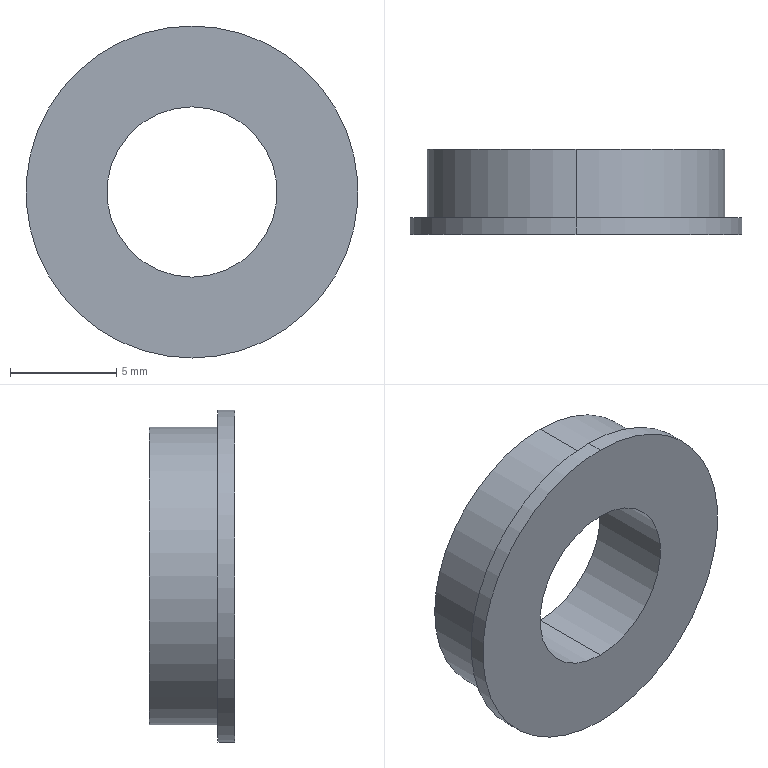Part | STEP file | Bearing 814 | 1 solid | 15 faces | box 15.6 x 4 x 15.6 mm | volume 433.486 mm3 | cylinder 10 | plane 5 | commonest cylinder face diameters 8 x2 9.644 x2 11.88 x2 14 x2 15.6 x2
STEP:
#1=CARTESIAN_POINT('',(0.,0.,0.));
#2=DIRECTION('',(0.,0.,1.));
#3=DIRECTION('',(1.,0.,0.));
#4=AXIS2_PLACEMENT_3D('',#1,#2,#3);
#5=CARTESIAN_POINT('',(0.,0.78,-7.8));
#6=VERTEX_POINT('',#5);
#7=CARTESIAN_POINT('',(0.,0.78,7.8));
#8=VERTEX_POINT('',#7);
#9=CARTESIAN_POINT('',(0.,0.78,0.));
#10=DIRECTION('',(0.,-1.,0.));
#11=DIRECTION('',(0.,0.,-1.));
#12=AXIS2_PLACEMENT_3D('',#9,#10,#11);
#13=CIRCLE('',#12,7.8);
#14=CARTESIAN_POINT('',(0.,0.,0.));
#15=DIRECTION('',(0.,-1.,0.));
#16=DIRECTION('',(0.,0.,-1.));
#17=AXIS2_PLACEMENT_3D('',#14,#15,#16);
#18=CYLINDRICAL_SURFACE('',#17,7.8);
#19=CARTESIAN_POINT('',(0.,-0.78));
#20=DIRECTION('',(1.,0.));
#21=VECTOR('',#20,1.);
#22=LINE('',#19,#21);
#23=(GEOMETRIC_REPRESENTATION_CONTEXT(2)PARAMETRIC_REPRESENTATION_CONTEXT()REPRESENTATION_CONTEXT('',''));
#24=DEFINITIONAL_REPRESENTATION('',(#22),#23);
#25=PCURVE('',#18,#24);
#26=CARTESIAN_POINT('',(7.,0.78,0.));
#27=DIRECTION('',(0.,1.,0.));
#28=DIRECTION('',(0.,0.,1.));
#29=AXIS2_PLACEMENT_3D('',#26,#27,#28);
#30=PLANE('',#29);
#31=CARTESIAN_POINT('',(-7.8,-7.));
#32=CARTESIAN_POINT('',(-7.8,6.51));
#33=CARTESIAN_POINT('',(3.9,-0.245));
#34=CARTESIAN_POINT('',(15.6,-7.));
#35=CARTESIAN_POINT('',(3.9,-13.755));
#36=CARTESIAN_POINT('',(-7.8,-20.51));
#37=CARTESIAN_POINT('',(-7.8,-7.));
#38=(BOUNDED_CURVE()B_SPLINE_CURVE(2,(#31,#32,#33,#34,#35,#36,#37),.UNSPECIFIED.,.T.,.F.)B_SPLINE_CURVE_WITH_KNOTS((1,2,2,2,2,1),(-2.094,0.,2.094,4.189,6.283,8.378),.UNSPECIFIED.)CURVE()GEOMETRIC_REPRESENTATION_ITEM()RATIONAL_B_SPLINE_CURVE((1.,0.5,1.,0.5,1.,0.5,1.))REPRESENTATION_ITEM(''));
#39=(GEOMETRIC_REPRESENTATION_CONTEXT(2)PARAMETRIC_REPRESENTATION_CONTEXT()REPRESENTATION_CONTEXT('',''));
#40=DEFINITIONAL_REPRESENTATION('',(#38),#39);
#41=PCURVE('',#30,#40);
#42=SURFACE_CURVE('',#13,(#25,#41),.PCURVE_S1.);
#43=EDGE_CURVE('',#6,#8,#42,.T.);
#44=ORIENTED_EDGE('',*,*,#43,.T.);
#45=CARTESIAN_POINT('',(0.,0.,7.8));
#46=VERTEX_POINT('',#45);
#47=CARTESIAN_POINT('',(0.,0.,7.8));
#48=DIRECTION('',(0.,-1.,0.));
#49=VECTOR('',#48,1.);
#50=LINE('',#47,#49);
#51=CARTESIAN_POINT('',(3.142,0.));
#52=DIRECTION('',(0.,1.));
#53=VECTOR('',#52,1.);
#54=LINE('',#51,#53);
#55=(GEOMETRIC_REPRESENTATION_CONTEXT(2)PARAMETRIC_REPRESENTATION_CONTEXT()REPRESENTATION_CONTEXT('',''));
#56=DEFINITIONAL_REPRESENTATION('',(#54),#55);
#57=PCURVE('',#18,#56);
#58=CARTESIAN_POINT('',(0.,0.,0.));
#59=DIRECTION('',(0.,-1.,0.));
#60=DIRECTION('',(0.,0.,-1.));
#61=AXIS2_PLACEMENT_3D('',#58,#59,#60);
#62=CYLINDRICAL_SURFACE('',#61,7.8);
#63=CARTESIAN_POINT('',(3.142,0.));
#64=DIRECTION('',(0.,1.));
#65=VECTOR('',#64,1.);
#66=LINE('',#63,#65);
#67=(GEOMETRIC_REPRESENTATION_CONTEXT(2)PARAMETRIC_REPRESENTATION_CONTEXT()REPRESENTATION_CONTEXT('',''));
#68=DEFINITIONAL_REPRESENTATION('',(#66),#67);
#69=PCURVE('',#62,#68);
#70=SURFACE_CURVE('',#50,(#57,#69),.PCURVE_S1.);
#71=EDGE_CURVE('',#8,#46,#70,.T.);
#72=ORIENTED_EDGE('',*,*,#71,.T.);
#73=CARTESIAN_POINT('',(0.,0.,-7.8));
#74=VERTEX_POINT('',#73);
#75=CARTESIAN_POINT('',(0.,0.,0.));
#76=DIRECTION('',(0.,-1.,0.));
#77=DIRECTION('',(0.,0.,-1.));
#78=AXIS2_PLACEMENT_3D('',#75,#76,#77);
#79=CIRCLE('',#78,7.8);
#80=CARTESIAN_POINT('',(0.,0.));
#81=DIRECTION('',(1.,0.));
#82=VECTOR('',#81,1.);
#83=LINE('',#80,#82);
#84=(GEOMETRIC_REPRESENTATION_CONTEXT(2)PARAMETRIC_REPRESENTATION_CONTEXT()REPRESENTATION_CONTEXT('',''));
#85=DEFINITIONAL_REPRESENTATION('',(#83),#84);
#86=PCURVE('',#18,#85);
#87=CARTESIAN_POINT('',(7.8,0.,0.));
#88=DIRECTION('',(0.,-1.,0.));
#89=DIRECTION('',(0.,0.,-1.));
#90=AXIS2_PLACEMENT_3D('',#87,#88,#89);
#91=PLANE('',#90);
#92=CARTESIAN_POINT('',(0.,-7.8));
#93=DIRECTION('',(1.,0.));
#94=AXIS2_PLACEMENT_2D('',#92,#93);
#95=CIRCLE('',#94,7.8);
#96=(GEOMETRIC_REPRESENTATION_CONTEXT(2)PARAMETRIC_REPRESENTATION_CONTEXT()REPRESENTATION_CONTEXT('',''));
#97=DEFINITIONAL_REPRESENTATION('',(#95),#96);
#98=PCURVE('',#91,#97);
#99=SURFACE_CURVE('',#79,(#86,#98),.PCURVE_S1.);
#100=EDGE_CURVE('',#74,#46,#99,.T.);
#101=ORIENTED_EDGE('',*,*,#100,.F.);
#102=CARTESIAN_POINT('',(0.,0.,-7.8));
#103=DIRECTION('',(0.,-1.,0.));
#104=VECTOR('',#103,1.);
#105=LINE('',#102,#104);
#106=CARTESIAN_POINT('',(0.,0.));
#107=DIRECTION('',(0.,1.));
#108=VECTOR('',#107,1.);
#109=LINE('',#106,#108);
#110=(GEOMETRIC_REPRESENTATION_CONTEXT(2)PARAMETRIC_REPRESENTATION_CONTEXT()REPRESENTATION_CONTEXT('',''));
#111=DEFINITIONAL_REPRESENTATION('',(#109),#110);
#112=PCURVE('',#18,#111);
#113=CARTESIAN_POINT('',(6.283,0.));
#114=DIRECTION('',(0.,1.));
#115=VECTOR('',#114,1.);
#116=LINE('',#113,#115);
#117=(GEOMETRIC_REPRESENTATION_CONTEXT(2)PARAMETRIC_REPRESENTATION_CONTEXT()REPRESENTATION_CONTEXT('',''));
#118=DEFINITIONAL_REPRESENTATION('',(#116),#117);
#119=PCURVE('',#62,#118);
#120=SURFACE_CURVE('',#105,(#112,#119),.PCURVE_S1.);
#121=EDGE_CURVE('',#6,#74,#120,.T.);
#122=ORIENTED_EDGE('',*,*,#121,.F.);
#123=EDGE_LOOP('',(#44,#72,#101,#122));
#124=FACE_BOUND('',#123,.T.);
#125=ADVANCED_FACE('',(#124),#18,.T.);
#126=CARTESIAN_POINT('',(0.,4.,-7.));
#127=VERTEX_POINT('',#126);
#128=CARTESIAN_POINT('',(0.,4.,7.));
#129=VERTEX_POINT('',#128);
#130=CARTESIAN_POINT('',(0.,4.,0.));
#131=DIRECTION('',(0.,-1.,0.));
#132=DIRECTION('',(0.,0.,-1.));
#133=AXIS2_PLACEMENT_3D('',#130,#131,#132);
#134=CIRCLE('',#133,7.);
#135=CARTESIAN_POINT('',(0.,0.,0.));
#136=DIRECTION('',(0.,-1.,0.));
#137=DIRECTION('',(0.,0.,-1.));
#138=AXIS2_PLACEMENT_3D('',#135,#136,#137);
#139=CYLINDRICAL_SURFACE('',#138,7.);
#140=CARTESIAN_POINT('',(0.,-4.));
#141=DIRECTION('',(1.,0.));
#142=VECTOR('',#141,1.);
#143=LINE('',#140,#142);
#144=(GEOMETRIC_REPRESENTATION_CONTEXT(2)PARAMETRIC_REPRESENTATION_CONTEXT()REPRESENTATION_CONTEXT('',''));
#145=DEFINITIONAL_REPRESENTATION('',(#143),#144);
#146=PCURVE('',#139,#145);
#147=CARTESIAN_POINT('',(5.94,4.,0.));
#148=DIRECTION('',(0.,1.,0.));
#149=DIRECTION('',(0.,0.,1.));
#150=AXIS2_PLACEMENT_3D('',#147,#148,#149);
#151=PLANE('',#150);
#152=CARTESIAN_POINT('',(-7.,-5.94));
#153=CARTESIAN_POINT('',(-7.,6.184));
#154=CARTESIAN_POINT('',(3.5,0.1221));
#155=CARTESIAN_POINT('',(14.,-5.94));
#156=CARTESIAN_POINT('',(3.5,-12.002));
#157=CARTESIAN_POINT('',(-7.,-18.064));
#158=CARTESIAN_POINT('',(-7.,-5.94));
#159=(BOUNDED_CURVE()B_SPLINE_CURVE(2,(#152,#153,#154,#155,#156,#157,#158),.UNSPECIFIED.,.T.,.F.)B_SPLINE_CURVE_WITH_KNOTS((1,2,2,2,2,1),(-2.094,0.,2.094,4.189,6.283,8.378),.UNSPECIFIED.)CURVE()GEOMETRIC_REPRESENTATION_ITEM()RATIONAL_B_SPLINE_CURVE((1.,0.5,1.,0.5,1.,0.5,1.))REPRESENTATION_ITEM(''));
#160=(GEOMETRIC_REPRESENTATION_CONTEXT(2)PARAMETRIC_REPRESENTATION_CONTEXT()REPRESENTATION_CONTEXT('',''));
#161=DEFINITIONAL_REPRESENTATION('',(#159),#160);
#162=PCURVE('',#151,#161);
#163=SURFACE_CURVE('',#134,(#146,#162),.PCURVE_S1.);
#164=EDGE_CURVE('',#127,#129,#163,.T.);
#165=ORIENTED_EDGE('',*,*,#164,.T.);
#166=CARTESIAN_POINT('',(0.,0.78,7.));
#167=VERTEX_POINT('',#166);
#168=CARTESIAN_POINT('',(0.,0.,7.));
#169=DIRECTION('',(0.,-1.,0.));
#170=VECTOR('',#169,1.);
#171=LINE('',#168,#170);
#172=CARTESIAN_POINT('',(3.142,0.));
#173=DIRECTION('',(0.,1.));
#174=VECTOR('',#173,1.);
#175=LINE('',#172,#174);
#176=(GEOMETRIC_REPRESENTATION_CONTEXT(2)PARAMETRIC_REPRESENTATION_CONTEXT()REPRESENTATION_CONTEXT('',''));
#177=DEFINITIONAL_REPRESENTATION('',(#175),#176);
#178=PCURVE('',#139,#177);
#179=CARTESIAN_POINT('',(0.,0.,0.));
#180=DIRECTION('',(0.,-1.,0.));
#181=DIRECTION('',(0.,0.,-1.));
#182=AXIS2_PLACEMENT_3D('',#179,#180,#181);
#183=CYLINDRICAL_SURFACE('',#182,7.);
#184=CARTESIAN_POINT('',(3.142,0.));
#185=DIRECTION('',(0.,1.));
#186=VECTOR('',#185,1.);
#187=LINE('',#184,#186);
#188=(GEOMETRIC_REPRESENTATION_CONTEXT(2)PARAMETRIC_REPRESENTATION_CONTEXT()REPRESENTATION_CONTEXT('',''));
#189=DEFINITIONAL_REPRESENTATION('',(#187),#188);
#190=PCURVE('',#183,#189);
#191=SURFACE_CURVE('',#171,(#178,#190),.PCURVE_S1.);
#192=EDGE_CURVE('',#129,#167,#191,.T.);
#193=ORIENTED_EDGE('',*,*,#192,.T.);
#194=CARTESIAN_POINT('',(0.,0.78,-7.));
#195=VERTEX_POINT('',#194);
#196=CARTESIAN_POINT('',(0.,0.78,0.));
#197=DIRECTION('',(0.,-1.,0.));
#198=DIRECTION('',(0.,0.,-1.));
#199=AXIS2_PLACEMENT_3D('',#196,#197,#198);
#200=CIRCLE('',#199,7.);
#201=CARTESIAN_POINT('',(0.,-0.78));
#202=DIRECTION('',(1.,0.));
#203=VECTOR('',#202,1.);
#204=LINE('',#201,#203);
#205=(GEOMETRIC_REPRESENTATION_CONTEXT(2)PARAMETRIC_REPRESENTATION_CONTEXT()REPRESENTATION_CONTEXT('',''));
#206=DEFINITIONAL_REPRESENTATION('',(#204),#205);
#207=PCURVE('',#139,#206);
#208=CARTESIAN_POINT('',(-7.,-7.));
#209=CARTESIAN_POINT('',(-7.,5.124));
#210=CARTESIAN_POINT('',(3.5,-0.9378));
#211=CARTESIAN_POINT('',(14.,-7.));
#212=CARTESIAN_POINT('',(3.5,-13.062));
#213=CARTESIAN_POINT('',(-7.,-19.124));
#214=CARTESIAN_POINT('',(-7.,-7.));
#215=(BOUNDED_CURVE()B_SPLINE_CURVE(2,(#208,#209,#210,#211,#212,#213,#214),.UNSPECIFIED.,.T.,.F.)B_SPLINE_CURVE_WITH_KNOTS((1,2,2,2,2,1),(-2.094,0.,2.094,4.189,6.283,8.378),.UNSPECIFIED.)CURVE()GEOMETRIC_REPRESENTATION_ITEM()RATIONAL_B_SPLINE_CURVE((1.,0.5,1.,0.5,1.,0.5,1.))REPRESENTATION_ITEM(''));
#216=(GEOMETRIC_REPRESENTATION_CONTEXT(2)PARAMETRIC_REPRESENTATION_CONTEXT()REPRESENTATION_CONTEXT('',''));
#217=DEFINITIONAL_REPRESENTATION('',(#215),#216);
#218=PCURVE('',#30,#217);
#219=SURFACE_CURVE('',#200,(#207,#218),.PCURVE_S1.);
#220=EDGE_CURVE('',#195,#167,#219,.T.);
#221=ORIENTED_EDGE('',*,*,#220,.F.);
#222=CARTESIAN_POINT('',(0.,0.,-7.));
#223=DIRECTION('',(0.,-1.,0.));
#224=VECTOR('',#223,1.);
#225=LINE('',#222,#224);
#226=CARTESIAN_POINT('',(0.,0.));
#227=DIRECTION('',(0.,1.));
#228=VECTOR('',#227,1.);
#229=LINE('',#226,#228);
#230=(GEOMETRIC_REPRESENTATION_CONTEXT(2)PARAMETRIC_REPRESENTATION_CONTEXT()REPRESENTATION_CONTEXT('',''));
#231=DEFINITIONAL_REPRESENTATION('',(#229),#230);
#232=PCURVE('',#139,#231);
#233=CARTESIAN_POINT('',(6.283,0.));
#234=DIRECTION('',(0.,1.));
#235=VECTOR('',#234,1.);
#236=LINE('',#233,#235);
#237=(GEOMETRIC_REPRESENTATION_CONTEXT(2)PARAMETRIC_REPRESENTATION_CONTEXT()REPRESENTATION_CONTEXT('',''));
#238=DEFINITIONAL_REPRESENTATION('',(#236),#237);
#239=PCURVE('',#183,#238);
#240=SURFACE_CURVE('',#225,(#232,#239),.PCURVE_S1.);
#241=EDGE_CURVE('',#127,#195,#240,.T.);
#242=ORIENTED_EDGE('',*,*,#241,.F.);
#243=EDGE_LOOP('',(#165,#193,#221,#242));
#244=FACE_BOUND('',#243,.T.);
#245=ADVANCED_FACE('',(#244),#139,.T.);
#246=CARTESIAN_POINT('',(0.,4.,-5.94));
#247=VERTEX_POINT('',#246);
#248=CARTESIAN_POINT('',(0.,3.73,-5.94));
#249=VERTEX_POINT('',#248);
#250=CARTESIAN_POINT('',(0.,0.,-5.94));
#251=DIRECTION('',(0.,-1.,0.));
#252=VECTOR('',#251,1.);
#253=LINE('',#250,#252);
#254=CARTESIAN_POINT('',(0.,0.,0.));
#255=DIRECTION('',(0.,-1.,0.));
#256=DIRECTION('',(0.,0.,-1.));
#257=AXIS2_PLACEMENT_3D('',#254,#255,#256);
#258=CYLINDRICAL_SURFACE('',#257,5.94);
#259=CARTESIAN_POINT('',(6.283,0.));
#260=DIRECTION('',(0.,1.));
#261=VECTOR('',#260,1.);
#262=LINE('',#259,#261);
#263=(GEOMETRIC_REPRESENTATION_CONTEXT(2)PARAMETRIC_REPRESENTATION_CONTEXT()REPRESENTATION_CONTEXT('',''));
#264=DEFINITIONAL_REPRESENTATION('',(#262),#263);
#265=PCURVE('',#258,#264);
#266=CARTESIAN_POINT('',(0.,0.,0.));
#267=DIRECTION('',(0.,-1.,0.));
#268=DIRECTION('',(0.,0.,-1.));
#269=AXIS2_PLACEMENT_3D('',#266,#267,#268);
#270=CYLINDRICAL_SURFACE('',#269,5.94);
#271=CARTESIAN_POINT('',(0.,0.));
#272=DIRECTION('',(0.,1.));
#273=VECTOR('',#272,1.);
#274=LINE('',#271,#273);
#275=(GEOMETRIC_REPRESENTATION_CONTEXT(2)PARAMETRIC_REPRESENTATION_CONTEXT()REPRESENTATION_CONTEXT('',''));
#276=DEFINITIONAL_REPRESENTATION('',(#274),#275);
#277=PCURVE('',#270,#276);
#278=SURFACE_CURVE('',#253,(#265,#277),.PCURVE_S1.);
#279=EDGE_CURVE('',#247,#249,#278,.T.);
#280=ORIENTED_EDGE('',*,*,#279,.T.);
#281=CARTESIAN_POINT('',(0.,3.73,5.94));
#282=VERTEX_POINT('',#281);
#283=CARTESIAN_POINT('',(0.,3.73,0.));
#284=DIRECTION('',(0.,-1.,0.));
#285=DIRECTION('',(0.,0.,-1.));
#286=AXIS2_PLACEMENT_3D('',#283,#284,#285);
#287=CIRCLE('',#286,5.94);
#288=CARTESIAN_POINT('',(0.,-3.73));
#289=DIRECTION('',(1.,0.));
#290=VECTOR('',#289,1.);
#291=LINE('',#288,#290);
#292=(GEOMETRIC_REPRESENTATION_CONTEXT(2)PARAMETRIC_REPRESENTATION_CONTEXT()REPRESENTATION_CONTEXT('',''));
#293=DEFINITIONAL_REPRESENTATION('',(#291),#292);
#294=PCURVE('',#258,#293);
#295=CARTESIAN_POINT('',(5.383,3.73,0.));
#296=DIRECTION('',(0.,1.,0.));
#297=DIRECTION('',(0.,0.,1.));
#298=AXIS2_PLACEMENT_3D('',#295,#296,#297);
#299=PLANE('',#298);
#300=CARTESIAN_POINT('',(-5.94,-5.383));
#301=CARTESIAN_POINT('',(-5.94,4.906));
#302=CARTESIAN_POINT('',(2.97,-0.2387));
#303=CARTESIAN_POINT('',(11.88,-5.383));
#304=CARTESIAN_POINT('',(2.97,-10.527));
#305=CARTESIAN_POINT('',(-5.94,-15.672));
#306=CARTESIAN_POINT('',(-5.94,-5.383));
#307=(BOUNDED_CURVE()B_SPLINE_CURVE(2,(#300,#301,#302,#303,#304,#305,#306),.UNSPECIFIED.,.T.,.F.)B_SPLINE_CURVE_WITH_KNOTS((1,2,2,2,2,1),(-2.094,0.,2.094,4.189,6.283,8.378),.UNSPECIFIED.)CURVE()GEOMETRIC_REPRESENTATION_ITEM()RATIONAL_B_SPLINE_CURVE((1.,0.5,1.,0.5,1.,0.5,1.))REPRESENTATION_ITEM(''));
#308=(GEOMETRIC_REPRESENTATION_CONTEXT(2)PARAMETRIC_REPRESENTATION_CONTEXT()REPRESENTATION_CONTEXT('',''));
#309=DEFINITIONAL_REPRESENTATION('',(#307),#308);
#310=PCURVE('',#299,#309);
#311=SURFACE_CURVE('',#287,(#294,#310),.PCURVE_S1.);
#312=EDGE_CURVE('',#282,#249,#311,.T.);
#313=ORIENTED_EDGE('',*,*,#312,.F.);
#314=CARTESIAN_POINT('',(0.,4.,5.94));
#315=VERTEX_POINT('',#314);
#316=CARTESIAN_POINT('',(0.,0.,5.94));
#317=DIRECTION('',(0.,-1.,0.));
#318=VECTOR('',#317,1.);
#319=LINE('',#316,#318);
#320=CARTESIAN_POINT('',(3.142,0.));
#321=DIRECTION('',(0.,1.));
#322=VECTOR('',#321,1.);
#323=LINE('',#320,#322);
#324=(GEOMETRIC_REPRESENTATION_CONTEXT(2)PARAMETRIC_REPRESENTATION_CONTEXT()REPRESENTATION_CONTEXT('',''));
#325=DEFINITIONAL_REPRESENTATION('',(#323),#324);
#326=PCURVE('',#258,#325);
#327=CARTESIAN_POINT('',(3.142,0.));
#328=DIRECTION('',(0.,1.));
#329=VECTOR('',#328,1.);
#330=LINE('',#327,#329);
#331=(GEOMETRIC_REPRESENTATION_CONTEXT(2)PARAMETRIC_REPRESENTATION_CONTEXT()REPRESENTATION_CONTEXT('',''));
#332=DEFINITIONAL_REPRESENTATION('',(#330),#331);
#333=PCURVE('',#270,#332);
#334=SURFACE_CURVE('',#319,(#326,#333),.PCURVE_S1.);
#335=EDGE_CURVE('',#315,#282,#334,.T.);
#336=ORIENTED_EDGE('',*,*,#335,.F.);
#337=CARTESIAN_POINT('',(0.,4.,0.));
#338=DIRECTION('',(0.,-1.,0.));
#339=DIRECTION('',(0.,0.,-1.));
#340=AXIS2_PLACEMENT_3D('',#337,#338,#339);
#341=CIRCLE('',#340,5.94);
#342=CARTESIAN_POINT('',(0.,-4.));
#343=DIRECTION('',(1.,0.));
#344=VECTOR('',#343,1.);
#345=LINE('',#342,#344);
#346=(GEOMETRIC_REPRESENTATION_CONTEXT(2)PARAMETRIC_REPRESENTATION_CONTEXT()REPRESENTATION_CONTEXT('',''));
#347=DEFINITIONAL_REPRESENTATION('',(#345),#346);
#348=PCURVE('',#258,#347);
#349=CARTESIAN_POINT('',(-5.94,-5.94));
#350=CARTESIAN_POINT('',(-5.94,4.348));
#351=CARTESIAN_POINT('',(2.97,-0.7958));
#352=CARTESIAN_POINT('',(11.88,-5.94));
#353=CARTESIAN_POINT('',(2.97,-11.084));
#354=CARTESIAN_POINT('',(-5.94,-16.229));
#355=CARTESIAN_POINT('',(-5.94,-5.94));
#356=(BOUNDED_CURVE()B_SPLINE_CURVE(2,(#349,#350,#351,#352,#353,#354,#355),.UNSPECIFIED.,.T.,.F.)B_SPLINE_CURVE_WITH_KNOTS((1,2,2,2,2,1),(-2.094,0.,2.094,4.189,6.283,8.378),.UNSPECIFIED.)CURVE()GEOMETRIC_REPRESENTATION_ITEM()RATIONAL_B_SPLINE_CURVE((1.,0.5,1.,0.5,1.,0.5,1.))REPRESENTATION_ITEM(''));
#357=(GEOMETRIC_REPRESENTATION_CONTEXT(2)PARAMETRIC_REPRESENTATION_CONTEXT()REPRESENTATION_CONTEXT('',''));
#358=DEFINITIONAL_REPRESENTATION('',(#356),#357);
#359=PCURVE('',#151,#358);
#360=SURFACE_CURVE('',#341,(#348,#359),.PCURVE_S1.);
#361=EDGE_CURVE('',#315,#247,#360,.T.);
#362=ORIENTED_EDGE('',*,*,#361,.T.);
#363=EDGE_LOOP('',(#280,#313,#336,#362));
#364=FACE_BOUND('',#363,.F.);
#365=ADVANCED_FACE('',(#364),#258,.F.);
#366=CARTESIAN_POINT('',(0.,4.,-4.822));
#367=VERTEX_POINT('',#366);
#368=CARTESIAN_POINT('',(0.,4.,4.822));
#369=VERTEX_POINT('',#368);
#370=CARTESIAN_POINT('',(0.,4.,0.));
#371=DIRECTION('',(0.,-1.,0.));
#372=DIRECTION('',(0.,0.,-1.));
#373=AXIS2_PLACEMENT_3D('',#370,#371,#372);
#374=CIRCLE('',#373,4.822);
#375=CARTESIAN_POINT('',(0.,0.,0.));
#376=DIRECTION('',(0.,-1.,0.));
#377=DIRECTION('',(0.,0.,-1.));
#378=AXIS2_PLACEMENT_3D('',#375,#376,#377);
#379=CYLINDRICAL_SURFACE('',#378,4.822);
#380=CARTESIAN_POINT('',(0.,-4.));
#381=DIRECTION('',(1.,0.));
#382=VECTOR('',#381,1.);
#383=LINE('',#380,#382);
#384=(GEOMETRIC_REPRESENTATION_CONTEXT(2)PARAMETRIC_REPRESENTATION_CONTEXT()REPRESENTATION_CONTEXT('',''));
#385=DEFINITIONAL_REPRESENTATION('',(#383),#384);
#386=PCURVE('',#379,#385);
#387=CARTESIAN_POINT('',(4.,4.,0.));
#388=DIRECTION('',(0.,1.,0.));
#389=DIRECTION('',(0.,0.,1.));
#390=AXIS2_PLACEMENT_3D('',#387,#388,#389);
#391=PLANE('',#390);
#392=CARTESIAN_POINT('',(-4.822,-4.));
#393=CARTESIAN_POINT('',(-4.822,4.352));
#394=CARTESIAN_POINT('',(2.411,0.1758));
#395=CARTESIAN_POINT('',(9.644,-4.));
#396=CARTESIAN_POINT('',(2.411,-8.176));
#397=CARTESIAN_POINT('',(-4.822,-12.352));
#398=CARTESIAN_POINT('',(-4.822,-4.));
#399=(BOUNDED_CURVE()B_SPLINE_CURVE(2,(#392,#393,#394,#395,#396,#397,#398),.UNSPECIFIED.,.T.,.F.)B_SPLINE_CURVE_WITH_KNOTS((1,2,2,2,2,1),(-2.094,0.,2.094,4.189,6.283,8.378),.UNSPECIFIED.)CURVE()GEOMETRIC_REPRESENTATION_ITEM()RATIONAL_B_SPLINE_CURVE((1.,0.5,1.,0.5,1.,0.5,1.))REPRESENTATION_ITEM(''));
#400=(GEOMETRIC_REPRESENTATION_CONTEXT(2)PARAMETRIC_REPRESENTATION_CONTEXT()REPRESENTATION_CONTEXT('',''));
#401=DEFINITIONAL_REPRESENTATION('',(#399),#400);
#402=PCURVE('',#391,#401);
#403=SURFACE_CURVE('',#374,(#386,#402),.PCURVE_S1.);
#404=EDGE_CURVE('',#367,#369,#403,.T.);
#405=ORIENTED_EDGE('',*,*,#404,.T.);
#406=CARTESIAN_POINT('',(0.,3.73,4.822));
#407=VERTEX_POINT('',#406);
#408=CARTESIAN_POINT('',(0.,0.,4.822));
#409=DIRECTION('',(0.,-1.,0.));
#410=VECTOR('',#409,1.);
#411=LINE('',#408,#410);
#412=CARTESIAN_POINT('',(3.142,0.));
#413=DIRECTION('',(0.,1.));
#414=VECTOR('',#413,1.);
#415=LINE('',#412,#414);
#416=(GEOMETRIC_REPRESENTATION_CONTEXT(2)PARAMETRIC_REPRESENTATION_CONTEXT()REPRESENTATION_CONTEXT('',''));
#417=DEFINITIONAL_REPRESENTATION('',(#415),#416);
#418=PCURVE('',#379,#417);
#419=CARTESIAN_POINT('',(0.,0.,0.));
#420=DIRECTION('',(0.,-1.,0.));
#421=DIRECTION('',(0.,0.,-1.));
#422=AXIS2_PLACEMENT_3D('',#419,#420,#421);
#423=CYLINDRICAL_SURFACE('',#422,4.822);
#424=CARTESIAN_POINT('',(3.142,0.));
#425=DIRECTION('',(0.,1.));
#426=VECTOR('',#425,1.);
#427=LINE('',#424,#426);
#428=(GEOMETRIC_REPRESENTATION_CONTEXT(2)PARAMETRIC_REPRESENTATION_CONTEXT()REPRESENTATION_CONTEXT('',''));
#429=DEFINITIONAL_REPRESENTATION('',(#427),#428);
#430=PCURVE('',#423,#429);
#431=SURFACE_CURVE('',#411,(#418,#430),.PCURVE_S1.);
#432=EDGE_CURVE('',#369,#407,#431,.T.);
#433=ORIENTED_EDGE('',*,*,#432,.T.);
#434=CARTESIAN_POINT('',(0.,3.73,-4.822));
#435=VERTEX_POINT('',#434);
#436=CARTESIAN_POINT('',(0.,3.73,0.));
#437=DIRECTION('',(0.,-1.,0.));
#438=DIRECTION('',(0.,0.,-1.));
#439=AXIS2_PLACEMENT_3D('',#436,#437,#438);
#440=CIRCLE('',#439,4.822);
#441=CARTESIAN_POINT('',(0.,-3.73));
#442=DIRECTION('',(1.,0.));
#443=VECTOR('',#442,1.);
#444=LINE('',#441,#443);
#445=(GEOMETRIC_REPRESENTATION_CONTEXT(2)PARAMETRIC_REPRESENTATION_CONTEXT()REPRESENTATION_CONTEXT('',''));
#446=DEFINITIONAL_REPRESENTATION('',(#444),#445);
#447=PCURVE('',#379,#446);
#448=CARTESIAN_POINT('',(-4.822,-5.383));
#449=CARTESIAN_POINT('',(-4.822,2.969));
#450=CARTESIAN_POINT('',(2.411,-1.207));
#451=CARTESIAN_POINT('',(9.644,-5.383));
#452=CARTESIAN_POINT('',(2.411,-9.559));
#453=CARTESIAN_POINT('',(-4.822,-13.735));
#454=CARTESIAN_POINT('',(-4.822,-5.383));
#455=(BOUNDED_CURVE()B_SPLINE_CURVE(2,(#448,#449,#450,#451,#452,#453,#454),.UNSPECIFIED.,.T.,.F.)B_SPLINE_CURVE_WITH_KNOTS((1,2,2,2,2,1),(-2.094,0.,2.094,4.189,6.283,8.378),.UNSPECIFIED.)CURVE()GEOMETRIC_REPRESENTATION_ITEM()RATIONAL_B_SPLINE_CURVE((1.,0.5,1.,0.5,1.,0.5,1.))REPRESENTATION_ITEM(''));
#456=(GEOMETRIC_REPRESENTATION_CONTEXT(2)PARAMETRIC_REPRESENTATION_CONTEXT()REPRESENTATION_CONTEXT('',''));
#457=DEFINITIONAL_REPRESENTATION('',(#455),#456);
#458=PCURVE('',#299,#457);
#459=SURFACE_CURVE('',#440,(#447,#458),.PCURVE_S1.);
#460=EDGE_CURVE('',#435,#407,#459,.T.);
#461=ORIENTED_EDGE('',*,*,#460,.F.);
#462=CARTESIAN_POINT('',(0.,0.,-4.822));
#463=DIRECTION('',(0.,-1.,0.));
#464=VECTOR('',#463,1.);
#465=LINE('',#462,#464);
#466=CARTESIAN_POINT('',(0.,0.));
#467=DIRECTION('',(0.,1.));
#468=VECTOR('',#467,1.);
#469=LINE('',#466,#468);
#470=(GEOMETRIC_REPRESENTATION_CONTEXT(2)PARAMETRIC_REPRESENTATION_CONTEXT()REPRESENTATION_CONTEXT('',''));
#471=DEFINITIONAL_REPRESENTATION('',(#469),#470);
#472=PCURVE('',#379,#471);
#473=CARTESIAN_POINT('',(6.283,0.));
#474=DIRECTION('',(0.,1.));
#475=VECTOR('',#474,1.);
#476=LINE('',#473,#475);
#477=(GEOMETRIC_REPRESENTATION_CONTEXT(2)PARAMETRIC_REPRESENTATION_CONTEXT()REPRESENTATION_CONTEXT('',''));
#478=DEFINITIONAL_REPRESENTATION('',(#476),#477);
#479=PCURVE('',#423,#478);
#480=SURFACE_CURVE('',#465,(#472,#479),.PCURVE_S1.);
#481=EDGE_CURVE('',#367,#435,#480,.T.);
#482=ORIENTED_EDGE('',*,*,#481,.F.);
#483=EDGE_LOOP('',(#405,#433,#461,#482));
#484=FACE_BOUND('',#483,.T.);
#485=ADVANCED_FACE('',(#484),#379,.T.);
#486=CARTESIAN_POINT('',(0.,4.,-4.));
#487=VERTEX_POINT('',#486);
#488=CARTESIAN_POINT('',(0.,0.,-4.));
#489=VERTEX_POINT('',#488);
#490=CARTESIAN_POINT('',(0.,0.,-4.));
#491=DIRECTION('',(0.,-1.,0.));
#492=VECTOR('',#491,1.);
#493=LINE('',#490,#492);
#494=CARTESIAN_POINT('',(0.,0.,0.));
#495=DIRECTION('',(0.,-1.,0.));
#496=DIRECTION('',(0.,0.,-1.));
#497=AXIS2_PLACEMENT_3D('',#494,#495,#496);
#498=CYLINDRICAL_SURFACE('',#497,4.);
#499=CARTESIAN_POINT('',(6.283,0.));
#500=DIRECTION('',(0.,1.));
#501=VECTOR('',#500,1.);
#502=LINE('',#499,#501);
#503=(GEOMETRIC_REPRESENTATION_CONTEXT(2)PARAMETRIC_REPRESENTATION_CONTEXT()REPRESENTATION_CONTEXT('',''));
#504=DEFINITIONAL_REPRESENTATION('',(#502),#503);
#505=PCURVE('',#498,#504);
#506=CARTESIAN_POINT('',(0.,0.,0.));
#507=DIRECTION('',(0.,-1.,0.));
#508=DIRECTION('',(0.,0.,-1.));
#509=AXIS2_PLACEMENT_3D('',#506,#507,#508);
#510=CYLINDRICAL_SURFACE('',#509,4.);
#511=CARTESIAN_POINT('',(0.,0.));
#512=DIRECTION('',(0.,1.));
#513=VECTOR('',#512,1.);
#514=LINE('',#511,#513);
#515=(GEOMETRIC_REPRESENTATION_CONTEXT(2)PARAMETRIC_REPRESENTATION_CONTEXT()REPRESENTATION_CONTEXT('',''));
#516=DEFINITIONAL_REPRESENTATION('',(#514),#515);
#517=PCURVE('',#510,#516);
#518=SURFACE_CURVE('',#493,(#505,#517),.PCURVE_S1.);
#519=EDGE_CURVE('',#487,#489,#518,.T.);
#520=ORIENTED_EDGE('',*,*,#519,.T.);
#521=CARTESIAN_POINT('',(0.,0.,4.));
#522=VERTEX_POINT('',#521);
#523=CARTESIAN_POINT('',(0.,0.,0.));
#524=DIRECTION('',(0.,-1.,0.));
#525=DIRECTION('',(0.,0.,-1.));
#526=AXIS2_PLACEMENT_3D('',#523,#524,#525);
#527=CIRCLE('',#526,4.);
#528=CARTESIAN_POINT('',(0.,0.));
#529=DIRECTION('',(1.,0.));
#530=VECTOR('',#529,1.);
#531=LINE('',#528,#530);
#532=(GEOMETRIC_REPRESENTATION_CONTEXT(2)PARAMETRIC_REPRESENTATION_CONTEXT()REPRESENTATION_CONTEXT('',''));
#533=DEFINITIONAL_REPRESENTATION('',(#531),#532);
#534=PCURVE('',#498,#533);
#535=CARTESIAN_POINT('',(0.,-7.8));
#536=DIRECTION('',(1.,0.));
#537=AXIS2_PLACEMENT_2D('',#535,#536);
#538=CIRCLE('',#537,4.);
#539=(GEOMETRIC_REPRESENTATION_CONTEXT(2)PARAMETRIC_REPRESENTATION_CONTEXT()REPRESENTATION_CONTEXT('',''));
#540=DEFINITIONAL_REPRESENTATION('',(#538),#539);
#541=PCURVE('',#91,#540);
#542=SURFACE_CURVE('',#527,(#534,#541),.PCURVE_S1.);
#543=EDGE_CURVE('',#522,#489,#542,.T.);
#544=ORIENTED_EDGE('',*,*,#543,.F.);
#545=CARTESIAN_POINT('',(0.,4.,4.));
#546=VERTEX_POINT('',#545);
#547=CARTESIAN_POINT('',(0.,0.,4.));
#548=DIRECTION('',(0.,-1.,0.));
#549=VECTOR('',#548,1.);
#550=LINE('',#547,#549);
#551=CARTESIAN_POINT('',(3.142,0.));
#552=DIRECTION('',(0.,1.));
#553=VECTOR('',#552,1.);
#554=LINE('',#551,#553);
#555=(GEOMETRIC_REPRESENTATION_CONTEXT(2)PARAMETRIC_REPRESENTATION_CONTEXT()REPRESENTATION_CONTEXT('',''));
#556=DEFINITIONAL_REPRESENTATION('',(#554),#555);
#557=PCURVE('',#498,#556);
#558=CARTESIAN_POINT('',(3.142,0.));
#559=DIRECTION('',(0.,1.));
#560=VECTOR('',#559,1.);
#561=LINE('',#558,#560);
#562=(GEOMETRIC_REPRESENTATION_CONTEXT(2)PARAMETRIC_REPRESENTATION_CONTEXT()REPRESENTATION_CONTEXT('',''));
#563=DEFINITIONAL_REPRESENTATION('',(#561),#562);
#564=PCURVE('',#510,#563);
#565=SURFACE_CURVE('',#550,(#557,#564),.PCURVE_S1.);
#566=EDGE_CURVE('',#546,#522,#565,.T.);
#567=ORIENTED_EDGE('',*,*,#566,.F.);
#568=CARTESIAN_POINT('',(0.,4.,0.));
#569=DIRECTION('',(0.,-1.,0.));
#570=DIRECTION('',(0.,0.,-1.));
#571=AXIS2_PLACEMENT_3D('',#568,#569,#570);
#572=CIRCLE('',#571,4.);
#573=CARTESIAN_POINT('',(0.,-4.));
#574=DIRECTION('',(1.,0.));
#575=VECTOR('',#574,1.);
#576=LINE('',#573,#575);
#577=(GEOMETRIC_REPRESENTATION_CONTEXT(2)PARAMETRIC_REPRESENTATION_CONTEXT()REPRESENTATION_CONTEXT('',''));
#578=DEFINITIONAL_REPRESENTATION('',(#576),#577);
#579=PCURVE('',#498,#578);
#580=CARTESIAN_POINT('',(-4.,-4.));
#581=CARTESIAN_POINT('',(-4.,2.928));
#582=CARTESIAN_POINT('',(2.,-0.5359));
#583=CARTESIAN_POINT('',(8.,-4.));
#584=CARTESIAN_POINT('',(2.,-7.464));
#585=CARTESIAN_POINT('',(-4.,-10.928));
#586=CARTESIAN_POINT('',(-4.,-4.));
#587=(BOUNDED_CURVE()B_SPLINE_CURVE(2,(#580,#581,#582,#583,#584,#585,#586),.UNSPECIFIED.,.T.,.F.)B_SPLINE_CURVE_WITH_KNOTS((1,2,2,2,2,1),(-2.094,0.,2.094,4.189,6.283,8.378),.UNSPECIFIED.)CURVE()GEOMETRIC_REPRESENTATION_ITEM()RATIONAL_B_SPLINE_CURVE((1.,0.5,1.,0.5,1.,0.5,1.))REPRESENTATION_ITEM(''));
#588=(GEOMETRIC_REPRESENTATION_CONTEXT(2)PARAMETRIC_REPRESENTATION_CONTEXT()REPRESENTATION_CONTEXT('',''));
#589=DEFINITIONAL_REPRESENTATION('',(#587),#588);
#590=PCURVE('',#391,#589);
#591=SURFACE_CURVE('',#572,(#579,#590),.PCURVE_S1.);
#592=EDGE_CURVE('',#546,#487,#591,.T.);
#593=ORIENTED_EDGE('',*,*,#592,.T.);
#594=EDGE_LOOP('',(#520,#544,#567,#593));
#595=FACE_BOUND('',#594,.F.);
#596=ADVANCED_FACE('',(#595),#498,.F.);
#597=ORIENTED_EDGE('',*,*,#100,.T.);
#598=CARTESIAN_POINT('',(0.,0.,0.));
#599=DIRECTION('',(0.,-1.,0.));
#600=DIRECTION('',(0.,0.,-1.));
#601=AXIS2_PLACEMENT_3D('',#598,#599,#600);
#602=CIRCLE('',#601,7.8);
#603=CARTESIAN_POINT('',(0.,-7.8));
#604=DIRECTION('',(1.,0.));
#605=AXIS2_PLACEMENT_2D('',#603,#604);
#606=CIRCLE('',#605,7.8);
#607=(GEOMETRIC_REPRESENTATION_CONTEXT(2)PARAMETRIC_REPRESENTATION_CONTEXT()REPRESENTATION_CONTEXT('',''));
#608=DEFINITIONAL_REPRESENTATION('',(#606),#607);
#609=PCURVE('',#91,#608);
#610=CARTESIAN_POINT('',(0.,0.));
#611=DIRECTION('',(1.,0.));
#612=VECTOR('',#611,1.);
#613=LINE('',#610,#612);
#614=(GEOMETRIC_REPRESENTATION_CONTEXT(2)PARAMETRIC_REPRESENTATION_CONTEXT()REPRESENTATION_CONTEXT('',''));
#615=DEFINITIONAL_REPRESENTATION('',(#613),#614);
#616=PCURVE('',#62,#615);
#617=SURFACE_CURVE('',#602,(#609,#616),.PCURVE_S1.);
#618=EDGE_CURVE('',#46,#74,#617,.T.);
#619=ORIENTED_EDGE('',*,*,#618,.T.);
#620=EDGE_LOOP('',(#597,#619));
#621=FACE_BOUND('',#620,.T.);
#622=CARTESIAN_POINT('',(0.,0.,0.));
#623=DIRECTION('',(0.,-1.,0.));
#624=DIRECTION('',(0.,0.,-1.));
#625=AXIS2_PLACEMENT_3D('',#622,#623,#624);
#626=CIRCLE('',#625,4.);
#627=CARTESIAN_POINT('',(0.,-7.8));
#628=DIRECTION('',(1.,0.));
#629=AXIS2_PLACEMENT_2D('',#627,#628);
#630=CIRCLE('',#629,4.);
#631=(GEOMETRIC_REPRESENTATION_CONTEXT(2)PARAMETRIC_REPRESENTATION_CONTEXT()REPRESENTATION_CONTEXT('',''));
#632=DEFINITIONAL_REPRESENTATION('',(#630),#631);
#633=PCURVE('',#91,#632);
#634=CARTESIAN_POINT('',(0.,0.));
#635=DIRECTION('',(1.,0.));
#636=VECTOR('',#635,1.);
#637=LINE('',#634,#636);
#638=(GEOMETRIC_REPRESENTATION_CONTEXT(2)PARAMETRIC_REPRESENTATION_CONTEXT()REPRESENTATION_CONTEXT('',''));
#639=DEFINITIONAL_REPRESENTATION('',(#637),#638);
#640=PCURVE('',#510,#639);
#641=SURFACE_CURVE('',#626,(#633,#640),.PCURVE_S1.);
#642=EDGE_CURVE('',#489,#522,#641,.T.);
#643=ORIENTED_EDGE('',*,*,#642,.F.);
#644=ORIENTED_EDGE('',*,*,#543,.F.);
#645=EDGE_LOOP('',(#643,#644));
#646=FACE_BOUND('',#645,.T.);
#647=ADVANCED_FACE('',(#621,#646),#91,.T.);
#648=ORIENTED_EDGE('',*,*,#642,.F.);
#649=ORIENTED_EDGE('',*,*,#519,.F.);
#650=CARTESIAN_POINT('',(0.,4.,0.));
#651=DIRECTION('',(0.,-1.,0.));
#652=DIRECTION('',(0.,0.,-1.));
#653=AXIS2_PLACEMENT_3D('',#650,#651,#652);
#654=CIRCLE('',#653,4.);
#655=CARTESIAN_POINT('',(0.,-4.));
#656=DIRECTION('',(1.,0.));
#657=VECTOR('',#656,1.);
#658=LINE('',#655,#657);
#659=(GEOMETRIC_REPRESENTATION_CONTEXT(2)PARAMETRIC_REPRESENTATION_CONTEXT()REPRESENTATION_CONTEXT('',''));
#660=DEFINITIONAL_REPRESENTATION('',(#658),#659);
#661=PCURVE('',#510,#660);
#662=CARTESIAN_POINT('',(-4.,-4.));
#663=CARTESIAN_POINT('',(-4.,2.928));
#664=CARTESIAN_POINT('',(2.,-0.5359));
#665=CARTESIAN_POINT('',(8.,-4.));
#666=CARTESIAN_POINT('',(2.,-7.464));
#667=CARTESIAN_POINT('',(-4.,-10.928));
#668=CARTESIAN_POINT('',(-4.,-4.));
#669=(BOUNDED_CURVE()B_SPLINE_CURVE(2,(#662,#663,#664,#665,#666,#667,#668),.UNSPECIFIED.,.T.,.F.)B_SPLINE_CURVE_WITH_KNOTS((1,2,2,2,2,1),(-2.094,0.,2.094,4.189,6.283,8.378),.UNSPECIFIED.)CURVE()GEOMETRIC_REPRESENTATION_ITEM()RATIONAL_B_SPLINE_CURVE((1.,0.5,1.,0.5,1.,0.5,1.))REPRESENTATION_ITEM(''));
#670=(GEOMETRIC_REPRESENTATION_CONTEXT(2)PARAMETRIC_REPRESENTATION_CONTEXT()REPRESENTATION_CONTEXT('',''));
#671=DEFINITIONAL_REPRESENTATION('',(#669),#670);
#672=PCURVE('',#391,#671);
#673=SURFACE_CURVE('',#654,(#661,#672),.PCURVE_S1.);
#674=EDGE_CURVE('',#487,#546,#673,.T.);
#675=ORIENTED_EDGE('',*,*,#674,.T.);
#676=ORIENTED_EDGE('',*,*,#566,.T.);
#677=EDGE_LOOP('',(#648,#649,#675,#676));
#678=FACE_BOUND('',#677,.F.);
#679=ADVANCED_FACE('',(#678),#510,.F.);
#680=ORIENTED_EDGE('',*,*,#674,.T.);
#681=ORIENTED_EDGE('',*,*,#592,.T.);
#682=EDGE_LOOP('',(#680,#681));
#683=FACE_BOUND('',#682,.T.);
#684=ORIENTED_EDGE('',*,*,#404,.F.);
#685=CARTESIAN_POINT('',(0.,4.,0.));
#686=DIRECTION('',(0.,-1.,0.));
#687=DIRECTION('',(0.,0.,-1.));
#688=AXIS2_PLACEMENT_3D('',#685,#686,#687);
#689=CIRCLE('',#688,4.822);
#690=CARTESIAN_POINT('',(-4.822,-4.));
#691=CARTESIAN_POINT('',(-4.822,4.352));
#692=CARTESIAN_POINT('',(2.411,0.1758));
#693=CARTESIAN_POINT('',(9.644,-4.));
#694=CARTESIAN_POINT('',(2.411,-8.176));
#695=CARTESIAN_POINT('',(-4.822,-12.352));
#696=CARTESIAN_POINT('',(-4.822,-4.));
#697=(BOUNDED_CURVE()B_SPLINE_CURVE(2,(#690,#691,#692,#693,#694,#695,#696),.UNSPECIFIED.,.T.,.F.)B_SPLINE_CURVE_WITH_KNOTS((1,2,2,2,2,1),(-2.094,0.,2.094,4.189,6.283,8.378),.UNSPECIFIED.)CURVE()GEOMETRIC_REPRESENTATION_ITEM()RATIONAL_B_SPLINE_CURVE((1.,0.5,1.,0.5,1.,0.5,1.))REPRESENTATION_ITEM(''));
#698=(GEOMETRIC_REPRESENTATION_CONTEXT(2)PARAMETRIC_REPRESENTATION_CONTEXT()REPRESENTATION_CONTEXT('',''));
#699=DEFINITIONAL_REPRESENTATION('',(#697),#698);
#700=PCURVE('',#391,#699);
#701=CARTESIAN_POINT('',(0.,-4.));
#702=DIRECTION('',(1.,0.));
#703=VECTOR('',#702,1.);
#704=LINE('',#701,#703);
#705=(GEOMETRIC_REPRESENTATION_CONTEXT(2)PARAMETRIC_REPRESENTATION_CONTEXT()REPRESENTATION_CONTEXT('',''));
#706=DEFINITIONAL_REPRESENTATION('',(#704),#705);
#707=PCURVE('',#423,#706);
#708=SURFACE_CURVE('',#689,(#700,#707),.PCURVE_S1.);
#709=EDGE_CURVE('',#369,#367,#708,.T.);
#710=ORIENTED_EDGE('',*,*,#709,.F.);
#711=EDGE_LOOP('',(#684,#710));
#712=FACE_BOUND('',#711,.T.);
#713=ADVANCED_FACE('',(#683,#712),#391,.T.);
#714=ORIENTED_EDGE('',*,*,#432,.F.);
#715=ORIENTED_EDGE('',*,*,#709,.T.);
#716=ORIENTED_EDGE('',*,*,#481,.T.);
#717=CARTESIAN_POINT('',(0.,3.73,0.));
#718=DIRECTION('',(0.,-1.,0.));
#719=DIRECTION('',(0.,0.,-1.));
#720=AXIS2_PLACEMENT_3D('',#717,#718,#719);
#721=CIRCLE('',#720,4.822);
#722=CARTESIAN_POINT('',(0.,-3.73));
#723=DIRECTION('',(1.,0.));
#724=VECTOR('',#723,1.);
#725=LINE('',#722,#724);
#726=(GEOMETRIC_REPRESENTATION_CONTEXT(2)PARAMETRIC_REPRESENTATION_CONTEXT()REPRESENTATION_CONTEXT('',''));
#727=DEFINITIONAL_REPRESENTATION('',(#725),#726);
#728=PCURVE('',#423,#727);
#729=CARTESIAN_POINT('',(-4.822,-5.383));
#730=CARTESIAN_POINT('',(-4.822,2.969));
#731=CARTESIAN_POINT('',(2.411,-1.207));
#732=CARTESIAN_POINT('',(9.644,-5.383));
#733=CARTESIAN_POINT('',(2.411,-9.559));
#734=CARTESIAN_POINT('',(-4.822,-13.735));
#735=CARTESIAN_POINT('',(-4.822,-5.383));
#736=(BOUNDED_CURVE()B_SPLINE_CURVE(2,(#729,#730,#731,#732,#733,#734,#735),.UNSPECIFIED.,.T.,.F.)B_SPLINE_CURVE_WITH_KNOTS((1,2,2,2,2,1),(-2.094,0.,2.094,4.189,6.283,8.378),.UNSPECIFIED.)CURVE()GEOMETRIC_REPRESENTATION_ITEM()RATIONAL_B_SPLINE_CURVE((1.,0.5,1.,0.5,1.,0.5,1.))REPRESENTATION_ITEM(''));
#737=(GEOMETRIC_REPRESENTATION_CONTEXT(2)PARAMETRIC_REPRESENTATION_CONTEXT()REPRESENTATION_CONTEXT('',''));
#738=DEFINITIONAL_REPRESENTATION('',(#736),#737);
#739=PCURVE('',#299,#738);
#740=SURFACE_CURVE('',#721,(#728,#739),.PCURVE_S1.);
#741=EDGE_CURVE('',#407,#435,#740,.T.);
#742=ORIENTED_EDGE('',*,*,#741,.F.);
#743=EDGE_LOOP('',(#714,#715,#716,#742));
#744=FACE_BOUND('',#743,.T.);
#745=ADVANCED_FACE('',(#744),#423,.T.);
#746=ORIENTED_EDGE('',*,*,#460,.T.);
#747=ORIENTED_EDGE('',*,*,#741,.T.);
#748=EDGE_LOOP('',(#746,#747));
#749=FACE_BOUND('',#748,.T.);
#750=CARTESIAN_POINT('',(0.,3.73,0.));
#751=DIRECTION('',(0.,-1.,0.));
#752=DIRECTION('',(0.,0.,-1.));
#753=AXIS2_PLACEMENT_3D('',#750,#751,#752);
#754=CIRCLE('',#753,5.94);
#755=CARTESIAN_POINT('',(-5.94,-5.383));
#756=CARTESIAN_POINT('',(-5.94,4.906));
#757=CARTESIAN_POINT('',(2.97,-0.2387));
#758=CARTESIAN_POINT('',(11.88,-5.383));
#759=CARTESIAN_POINT('',(2.97,-10.527));
#760=CARTESIAN_POINT('',(-5.94,-15.672));
#761=CARTESIAN_POINT('',(-5.94,-5.383));
#762=(BOUNDED_CURVE()B_SPLINE_CURVE(2,(#755,#756,#757,#758,#759,#760,#761),.UNSPECIFIED.,.T.,.F.)B_SPLINE_CURVE_WITH_KNOTS((1,2,2,2,2,1),(-2.094,0.,2.094,4.189,6.283,8.378),.UNSPECIFIED.)CURVE()GEOMETRIC_REPRESENTATION_ITEM()RATIONAL_B_SPLINE_CURVE((1.,0.5,1.,0.5,1.,0.5,1.))REPRESENTATION_ITEM(''));
#763=(GEOMETRIC_REPRESENTATION_CONTEXT(2)PARAMETRIC_REPRESENTATION_CONTEXT()REPRESENTATION_CONTEXT('',''));
#764=DEFINITIONAL_REPRESENTATION('',(#762),#763);
#765=PCURVE('',#299,#764);
#766=CARTESIAN_POINT('',(0.,-3.73));
#767=DIRECTION('',(1.,0.));
#768=VECTOR('',#767,1.);
#769=LINE('',#766,#768);
#770=(GEOMETRIC_REPRESENTATION_CONTEXT(2)PARAMETRIC_REPRESENTATION_CONTEXT()REPRESENTATION_CONTEXT('',''));
#771=DEFINITIONAL_REPRESENTATION('',(#769),#770);
#772=PCURVE('',#270,#771);
#773=SURFACE_CURVE('',#754,(#765,#772),.PCURVE_S1.);
#774=EDGE_CURVE('',#249,#282,#773,.T.);
#775=ORIENTED_EDGE('',*,*,#774,.F.);
#776=ORIENTED_EDGE('',*,*,#312,.F.);
#777=EDGE_LOOP('',(#775,#776));
#778=FACE_BOUND('',#777,.T.);
#779=ADVANCED_FACE('',(#749,#778),#299,.T.);
#780=ORIENTED_EDGE('',*,*,#774,.F.);
#781=ORIENTED_EDGE('',*,*,#279,.F.);
#782=CARTESIAN_POINT('',(0.,4.,0.));
#783=DIRECTION('',(0.,-1.,0.));
#784=DIRECTION('',(0.,0.,-1.));
#785=AXIS2_PLACEMENT_3D('',#782,#783,#784);
#786=CIRCLE('',#785,5.94);
#787=CARTESIAN_POINT('',(0.,-4.));
#788=DIRECTION('',(1.,0.));
#789=VECTOR('',#788,1.);
#790=LINE('',#787,#789);
#791=(GEOMETRIC_REPRESENTATION_CONTEXT(2)PARAMETRIC_REPRESENTATION_CONTEXT()REPRESENTATION_CONTEXT('',''));
#792=DEFINITIONAL_REPRESENTATION('',(#790),#791);
#793=PCURVE('',#270,#792);
#794=CARTESIAN_POINT('',(-5.94,-5.94));
#795=CARTESIAN_POINT('',(-5.94,4.348));
#796=CARTESIAN_POINT('',(2.97,-0.7958));
#797=CARTESIAN_POINT('',(11.88,-5.94));
#798=CARTESIAN_POINT('',(2.97,-11.084));
#799=CARTESIAN_POINT('',(-5.94,-16.229));
#800=CARTESIAN_POINT('',(-5.94,-5.94));
#801=(BOUNDED_CURVE()B_SPLINE_CURVE(2,(#794,#795,#796,#797,#798,#799,#800),.UNSPECIFIED.,.T.,.F.)B_SPLINE_CURVE_WITH_KNOTS((1,2,2,2,2,1),(-2.094,0.,2.094,4.189,6.283,8.378),.UNSPECIFIED.)CURVE()GEOMETRIC_REPRESENTATION_ITEM()RATIONAL_B_SPLINE_CURVE((1.,0.5,1.,0.5,1.,0.5,1.))REPRESENTATION_ITEM(''));
#802=(GEOMETRIC_REPRESENTATION_CONTEXT(2)PARAMETRIC_REPRESENTATION_CONTEXT()REPRESENTATION_CONTEXT('',''));
#803=DEFINITIONAL_REPRESENTATION('',(#801),#802);
#804=PCURVE('',#151,#803);
#805=SURFACE_CURVE('',#786,(#793,#804),.PCURVE_S1.);
#806=EDGE_CURVE('',#247,#315,#805,.T.);
#807=ORIENTED_EDGE('',*,*,#806,.T.);
#808=ORIENTED_EDGE('',*,*,#335,.T.);
#809=EDGE_LOOP('',(#780,#781,#807,#808));
#810=FACE_BOUND('',#809,.F.);
#811=ADVANCED_FACE('',(#810),#270,.F.);
#812=ORIENTED_EDGE('',*,*,#806,.T.);
#813=ORIENTED_EDGE('',*,*,#361,.T.);
#814=EDGE_LOOP('',(#812,#813));
#815=FACE_BOUND('',#814,.T.);
#816=ORIENTED_EDGE('',*,*,#164,.F.);
#817=CARTESIAN_POINT('',(0.,4.,0.));
#818=DIRECTION('',(0.,-1.,0.));
#819=DIRECTION('',(0.,0.,-1.));
#820=AXIS2_PLACEMENT_3D('',#817,#818,#819);
#821=CIRCLE('',#820,7.);
#822=CARTESIAN_POINT('',(-7.,-5.94));
#823=CARTESIAN_POINT('',(-7.,6.184));
#824=CARTESIAN_POINT('',(3.5,0.1221));
#825=CARTESIAN_POINT('',(14.,-5.94));
#826=CARTESIAN_POINT('',(3.5,-12.002));
#827=CARTESIAN_POINT('',(-7.,-18.064));
#828=CARTESIAN_POINT('',(-7.,-5.94));
#829=(BOUNDED_CURVE()B_SPLINE_CURVE(2,(#822,#823,#824,#825,#826,#827,#828),.UNSPECIFIED.,.T.,.F.)B_SPLINE_CURVE_WITH_KNOTS((1,2,2,2,2,1),(-2.094,0.,2.094,4.189,6.283,8.378),.UNSPECIFIED.)CURVE()GEOMETRIC_REPRESENTATION_ITEM()RATIONAL_B_SPLINE_CURVE((1.,0.5,1.,0.5,1.,0.5,1.))REPRESENTATION_ITEM(''));
#830=(GEOMETRIC_REPRESENTATION_CONTEXT(2)PARAMETRIC_REPRESENTATION_CONTEXT()REPRESENTATION_CONTEXT('',''));
#831=DEFINITIONAL_REPRESENTATION('',(#829),#830);
#832=PCURVE('',#151,#831);
#833=CARTESIAN_POINT('',(0.,-4.));
#834=DIRECTION('',(1.,0.));
#835=VECTOR('',#834,1.);
#836=LINE('',#833,#835);
#837=(GEOMETRIC_REPRESENTATION_CONTEXT(2)PARAMETRIC_REPRESENTATION_CONTEXT()REPRESENTATION_CONTEXT('',''));
#838=DEFINITIONAL_REPRESENTATION('',(#836),#837);
#839=PCURVE('',#183,#838);
#840=SURFACE_CURVE('',#821,(#832,#839),.PCURVE_S1.);
#841=EDGE_CURVE('',#129,#127,#840,.T.);
#842=ORIENTED_EDGE('',*,*,#841,.F.);
#843=EDGE_LOOP('',(#816,#842));
#844=FACE_BOUND('',#843,.T.);
#845=ADVANCED_FACE('',(#815,#844),#151,.T.);
#846=ORIENTED_EDGE('',*,*,#192,.F.);
#847=ORIENTED_EDGE('',*,*,#841,.T.);
#848=ORIENTED_EDGE('',*,*,#241,.T.);
#849=CARTESIAN_POINT('',(0.,0.78,0.));
#850=DIRECTION('',(0.,-1.,0.));
#851=DIRECTION('',(0.,0.,-1.));
#852=AXIS2_PLACEMENT_3D('',#849,#850,#851);
#853=CIRCLE('',#852,7.);
#854=CARTESIAN_POINT('',(0.,-0.78));
#855=DIRECTION('',(1.,0.));
#856=VECTOR('',#855,1.);
#857=LINE('',#854,#856);
#858=(GEOMETRIC_REPRESENTATION_CONTEXT(2)PARAMETRIC_REPRESENTATION_CONTEXT()REPRESENTATION_CONTEXT('',''));
#859=DEFINITIONAL_REPRESENTATION('',(#857),#858);
#860=PCURVE('',#183,#859);
#861=CARTESIAN_POINT('',(-7.,-7.));
#862=CARTESIAN_POINT('',(-7.,5.124));
#863=CARTESIAN_POINT('',(3.5,-0.9378));
#864=CARTESIAN_POINT('',(14.,-7.));
#865=CARTESIAN_POINT('',(3.5,-13.062));
#866=CARTESIAN_POINT('',(-7.,-19.124));
#867=CARTESIAN_POINT('',(-7.,-7.));
#868=(BOUNDED_CURVE()B_SPLINE_CURVE(2,(#861,#862,#863,#864,#865,#866,#867),.UNSPECIFIED.,.T.,.F.)B_SPLINE_CURVE_WITH_KNOTS((1,2,2,2,2,1),(-2.094,0.,2.094,4.189,6.283,8.378),.UNSPECIFIED.)CURVE()GEOMETRIC_REPRESENTATION_ITEM()RATIONAL_B_SPLINE_CURVE((1.,0.5,1.,0.5,1.,0.5,1.))REPRESENTATION_ITEM(''));
#869=(GEOMETRIC_REPRESENTATION_CONTEXT(2)PARAMETRIC_REPRESENTATION_CONTEXT()REPRESENTATION_CONTEXT('',''));
#870=DEFINITIONAL_REPRESENTATION('',(#868),#869);
#871=PCURVE('',#30,#870);
#872=SURFACE_CURVE('',#853,(#860,#871),.PCURVE_S1.);
#873=EDGE_CURVE('',#167,#195,#872,.T.);
#874=ORIENTED_EDGE('',*,*,#873,.F.);
#875=EDGE_LOOP('',(#846,#847,#848,#874));
#876=FACE_BOUND('',#875,.T.);
#877=ADVANCED_FACE('',(#876),#183,.T.);
#878=ORIENTED_EDGE('',*,*,#220,.T.);
#879=ORIENTED_EDGE('',*,*,#873,.T.);
#880=EDGE_LOOP('',(#878,#879));
#881=FACE_BOUND('',#880,.T.);
#882=ORIENTED_EDGE('',*,*,#43,.F.);
#883=CARTESIAN_POINT('',(0.,0.78,0.));
#884=DIRECTION('',(0.,-1.,0.));
#885=DIRECTION('',(0.,0.,-1.));
#886=AXIS2_PLACEMENT_3D('',#883,#884,#885);
#887=CIRCLE('',#886,7.8);
#888=CARTESIAN_POINT('',(-7.8,-7.));
#889=CARTESIAN_POINT('',(-7.8,6.51));
#890=CARTESIAN_POINT('',(3.9,-0.245));
#891=CARTESIAN_POINT('',(15.6,-7.));
#892=CARTESIAN_POINT('',(3.9,-13.755));
#893=CARTESIAN_POINT('',(-7.8,-20.51));
#894=CARTESIAN_POINT('',(-7.8,-7.));
#895=(BOUNDED_CURVE()B_SPLINE_CURVE(2,(#888,#889,#890,#891,#892,#893,#894),.UNSPECIFIED.,.T.,.F.)B_SPLINE_CURVE_WITH_KNOTS((1,2,2,2,2,1),(-2.094,0.,2.094,4.189,6.283,8.378),.UNSPECIFIED.)CURVE()GEOMETRIC_REPRESENTATION_ITEM()RATIONAL_B_SPLINE_CURVE((1.,0.5,1.,0.5,1.,0.5,1.))REPRESENTATION_ITEM(''));
#896=(GEOMETRIC_REPRESENTATION_CONTEXT(2)PARAMETRIC_REPRESENTATION_CONTEXT()REPRESENTATION_CONTEXT('',''));
#897=DEFINITIONAL_REPRESENTATION('',(#895),#896);
#898=PCURVE('',#30,#897);
#899=CARTESIAN_POINT('',(0.,-0.78));
#900=DIRECTION('',(1.,0.));
#901=VECTOR('',#900,1.);
#902=LINE('',#899,#901);
#903=(GEOMETRIC_REPRESENTATION_CONTEXT(2)PARAMETRIC_REPRESENTATION_CONTEXT()REPRESENTATION_CONTEXT('',''));
#904=DEFINITIONAL_REPRESENTATION('',(#902),#903);
#905=PCURVE('',#62,#904);
#906=SURFACE_CURVE('',#887,(#898,#905),.PCURVE_S1.);
#907=EDGE_CURVE('',#8,#6,#906,.T.);
#908=ORIENTED_EDGE('',*,*,#907,.F.);
#909=EDGE_LOOP('',(#882,#908));
#910=FACE_BOUND('',#909,.T.);
#911=ADVANCED_FACE('',(#881,#910),#30,.T.);
#912=ORIENTED_EDGE('',*,*,#71,.F.);
#913=ORIENTED_EDGE('',*,*,#907,.T.);
#914=ORIENTED_EDGE('',*,*,#121,.T.);
#915=ORIENTED_EDGE('',*,*,#618,.F.);
#916=EDGE_LOOP('',(#912,#913,#914,#915));
#917=FACE_BOUND('',#916,.T.);
#918=ADVANCED_FACE('',(#917),#62,.T.);
#919=CLOSED_SHELL('',(#125,#245,#365,#485,#596,#647,#679,#713,#745,#779,#811,#845,#877,#911,#918));
#920=MANIFOLD_SOLID_BREP('',#919);
#921=(LENGTH_UNIT()NAMED_UNIT(*)SI_UNIT(.MILLI.,.METRE.));
#922=UNCERTAINTY_MEASURE_WITH_UNIT(LENGTH_MEASURE(0.0000001),#921,'','');
#923=(NAMED_UNIT(*)PLANE_ANGLE_UNIT()SI_UNIT($,.RADIAN.));
#924=(NAMED_UNIT(*)SI_UNIT($,.STERADIAN.)SOLID_ANGLE_UNIT());
#925=(GEOMETRIC_REPRESENTATION_CONTEXT(3)GLOBAL_UNCERTAINTY_ASSIGNED_CONTEXT((#922))GLOBAL_UNIT_ASSIGNED_CONTEXT((#921,#923,#924))REPRESENTATION_CONTEXT('',''));
#926=ADVANCED_BREP_SHAPE_REPRESENTATION('',(#4,#920),#925);